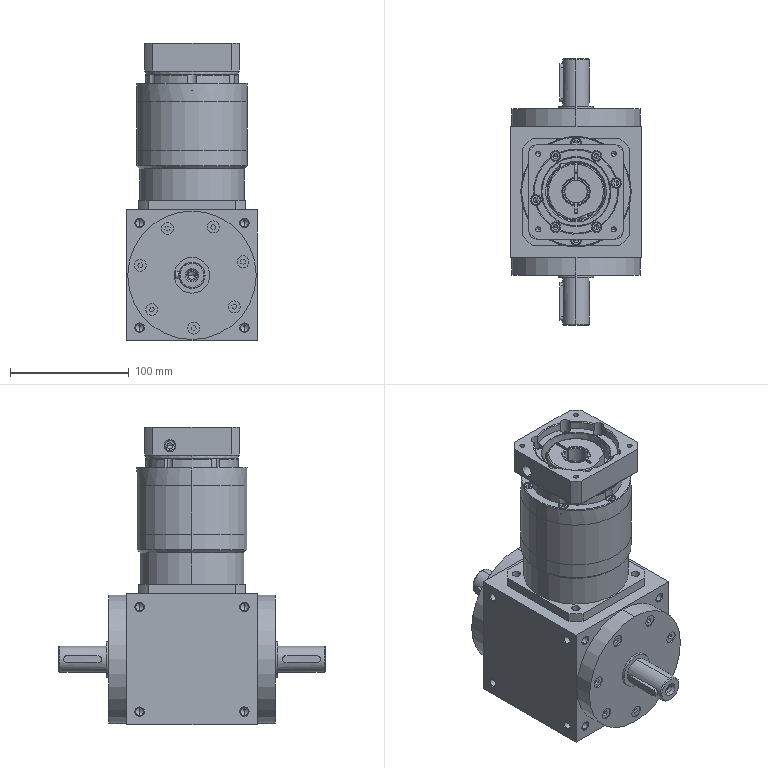Part | SolidWorks | features BaseBody 34 | 34 solids | 2230 faces | box 110 x 224 x 250 mm | volume 2228860 mm3 | spline 618 | plane 528 | cylinder 431 | cone 403 | torus 208 | sphere 42 | commonest cylinder face diameters 6.8 x84 4.2 x32 8.5 x28 10.003 x28 5 x26 9 x24